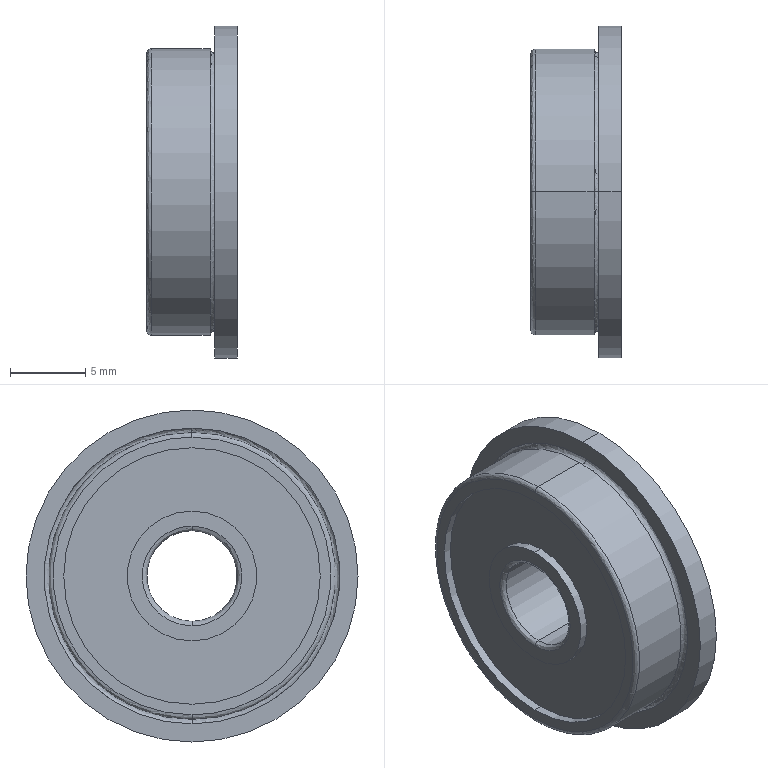Part | STEP file | Flanged ball bearing FL626ZZ | 1 solid | 29 faces | box 6 x 22 x 22 mm | volume 1471 mm3 | cylinder 14 | spline 8 | plane 7 | commonest cylinder face diameters 8.6 x4 17 x4 6 x2 19 x2 22 x2